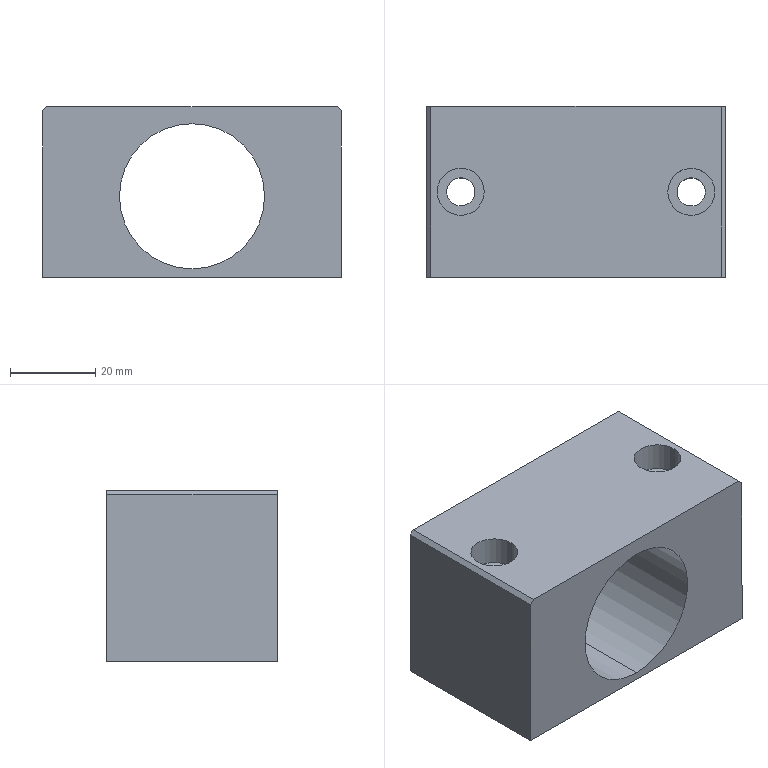Part | SolidWorks | features BaseBody 1 | 1 solid | 36 faces | box 70 x 40 x 40 mm | volume 71369 mm3 | cylinder 18 | plane 10 | cone 8 | commonest cylinder face diameters 4.2 x8 6.6 x4 11 x4 34 x2
STEP:
#1=CARTESIAN_POINT('',(-26.7,157.227,0.));
#2=VERTEX_POINT('',#1);
#3=CARTESIAN_POINT('',(-33.3,157.227,0.));
#4=VERTEX_POINT('',#3);
#5=CARTESIAN_POINT('',(-30.,157.227,0.));
#6=DIRECTION('',(0.,0.,-1.));
#7=DIRECTION('',(1.,0.,0.));
#8=AXIS2_PLACEMENT_3D('',#5,#6,#7);
#9=CIRCLE('',#8,3.3);
#10=EDGE_CURVE('',#2,#4,#9,.T.);
#11=ORIENTED_EDGE('',*,*,#10,.T.);
#12=CARTESIAN_POINT('',(-33.3,157.227,33.2));
#13=VERTEX_POINT('',#12);
#14=CARTESIAN_POINT('',(-33.3,157.227,40.));
#15=DIRECTION('',(0.,0.,1.));
#16=VECTOR('',#15,1000.);
#17=LINE('',#14,#16);
#18=EDGE_CURVE('',#4,#13,#17,.T.);
#19=ORIENTED_EDGE('',*,*,#18,.T.);
#20=CARTESIAN_POINT('',(-26.7,157.227,33.2));
#21=VERTEX_POINT('',#20);
#22=CARTESIAN_POINT('',(-30.,157.227,33.2));
#23=DIRECTION('',(0.,0.,-1.));
#24=DIRECTION('',(1.,0.,0.));
#25=AXIS2_PLACEMENT_3D('',#22,#23,#24);
#26=CIRCLE('',#25,3.3);
#27=EDGE_CURVE('',#21,#13,#26,.T.);
#28=ORIENTED_EDGE('',*,*,#27,.F.);
#29=CARTESIAN_POINT('',(-26.7,157.227,40.));
#30=DIRECTION('',(0.,0.,1.));
#31=VECTOR('',#30,1000.);
#32=LINE('',#29,#31);
#33=EDGE_CURVE('',#2,#21,#32,.T.);
#34=ORIENTED_EDGE('',*,*,#33,.F.);
#35=EDGE_LOOP('',(#11,#19,#28,#34));
#36=FACE_OUTER_BOUND('',#35,.T.);
#37=CARTESIAN_POINT('',(-30.,157.227,40.));
#38=DIRECTION('',(0.,0.,1.));
#39=DIRECTION('',(1.,0.,0.));
#40=AXIS2_PLACEMENT_3D('',#37,#38,#39);
#41=CYLINDRICAL_SURFACE('',#40,3.3);
#42=ADVANCED_FACE('',(#36),#41,.F.);
#43=CARTESIAN_POINT('',(27.3,157.184,0.));
#44=VERTEX_POINT('',#43);
#45=CARTESIAN_POINT('',(20.7,157.184,0.));
#46=VERTEX_POINT('',#45);
#47=CARTESIAN_POINT('',(24.,157.184,0.));
#48=DIRECTION('',(0.,0.,-1.));
#49=DIRECTION('',(1.,0.,0.));
#50=AXIS2_PLACEMENT_3D('',#47,#48,#49);
#51=CIRCLE('',#50,3.3);
#52=EDGE_CURVE('',#44,#46,#51,.T.);
#53=ORIENTED_EDGE('',*,*,#52,.T.);
#54=CARTESIAN_POINT('',(20.7,157.184,33.2));
#55=VERTEX_POINT('',#54);
#56=CARTESIAN_POINT('',(20.7,157.184,40.));
#57=DIRECTION('',(0.,0.,1.));
#58=VECTOR('',#57,1000.);
#59=LINE('',#56,#58);
#60=EDGE_CURVE('',#46,#55,#59,.T.);
#61=ORIENTED_EDGE('',*,*,#60,.T.);
#62=CARTESIAN_POINT('',(27.3,157.184,33.2));
#63=VERTEX_POINT('',#62);
#64=CARTESIAN_POINT('',(24.,157.184,33.2));
#65=DIRECTION('',(0.,0.,-1.));
#66=DIRECTION('',(1.,0.,0.));
#67=AXIS2_PLACEMENT_3D('',#64,#65,#66);
#68=CIRCLE('',#67,3.3);
#69=EDGE_CURVE('',#63,#55,#68,.T.);
#70=ORIENTED_EDGE('',*,*,#69,.F.);
#71=CARTESIAN_POINT('',(27.3,157.184,40.));
#72=DIRECTION('',(0.,0.,1.));
#73=VECTOR('',#72,1000.);
#74=LINE('',#71,#73);
#75=EDGE_CURVE('',#44,#63,#74,.T.);
#76=ORIENTED_EDGE('',*,*,#75,.F.);
#77=EDGE_LOOP('',(#53,#61,#70,#76));
#78=FACE_OUTER_BOUND('',#77,.T.);
#79=CARTESIAN_POINT('',(24.,157.184,40.));
#80=DIRECTION('',(0.,0.,1.));
#81=DIRECTION('',(1.,0.,0.));
#82=AXIS2_PLACEMENT_3D('',#79,#80,#81);
#83=CYLINDRICAL_SURFACE('',#82,3.3);
#84=ADVANCED_FACE('',(#78),#83,.F.);
#85=CARTESIAN_POINT('',(-3.,177.191,2.));
#86=VERTEX_POINT('',#85);
#87=CARTESIAN_POINT('',(-3.,177.191,36.));
#88=VERTEX_POINT('',#87);
#89=CARTESIAN_POINT('',(-3.,177.191,19.));
#90=DIRECTION('',(0.,1.,0.));
#91=DIRECTION('',(0.,0.,-1.));
#92=AXIS2_PLACEMENT_3D('',#89,#90,#91);
#93=CIRCLE('',#92,17.);
#94=EDGE_CURVE('',#86,#88,#93,.T.);
#95=ORIENTED_EDGE('',*,*,#94,.T.);
#96=CARTESIAN_POINT('',(-3.,137.191,36.));
#97=VERTEX_POINT('',#96);
#98=CARTESIAN_POINT('',(-3.,187.191,36.));
#99=DIRECTION('',(0.,-1.,0.));
#100=VECTOR('',#99,1000.);
#101=LINE('',#98,#100);
#102=EDGE_CURVE('',#88,#97,#101,.T.);
#103=ORIENTED_EDGE('',*,*,#102,.T.);
#104=CARTESIAN_POINT('',(-3.,137.191,2.));
#105=VERTEX_POINT('',#104);
#106=CARTESIAN_POINT('',(-3.,137.191,19.));
#107=DIRECTION('',(0.,-1.,0.));
#108=DIRECTION('',(0.,0.,-1.));
#109=AXIS2_PLACEMENT_3D('',#106,#107,#108);
#110=CIRCLE('',#109,17.);
#111=EDGE_CURVE('',#97,#105,#110,.T.);
#112=ORIENTED_EDGE('',*,*,#111,.T.);
#113=CARTESIAN_POINT('',(-3.,187.191,2.));
#114=DIRECTION('',(0.,-1.,0.));
#115=VECTOR('',#114,1000.);
#116=LINE('',#113,#115);
#117=EDGE_CURVE('',#86,#105,#116,.T.);
#118=ORIENTED_EDGE('',*,*,#117,.F.);
#119=EDGE_LOOP('',(#95,#103,#112,#118));
#120=FACE_OUTER_BOUND('',#119,.T.);
#121=CARTESIAN_POINT('',(-3.,187.191,19.));
#122=DIRECTION('',(0.,-1.,0.));
#123=DIRECTION('',(0.,0.,-1.));
#124=AXIS2_PLACEMENT_3D('',#121,#122,#123);
#125=CYLINDRICAL_SURFACE('',#124,17.);
#126=ADVANCED_FACE('',(#120),#125,.F.);
#127=CARTESIAN_POINT('',(-22.486,164.791,28.15));
#128=VERTEX_POINT('',#127);
#129=CARTESIAN_POINT('',(-22.486,164.791,32.35));
#130=VERTEX_POINT('',#129);
#131=CARTESIAN_POINT('',(-22.486,164.791,30.25));
#132=DIRECTION('',(0.,1.,0.));
#133=DIRECTION('',(0.,0.,1.));
#134=AXIS2_PLACEMENT_3D('',#131,#132,#133);
#135=CIRCLE('',#134,2.1);
#136=EDGE_CURVE('',#128,#130,#135,.T.);
#137=ORIENTED_EDGE('',*,*,#136,.F.);
#138=CARTESIAN_POINT('',(-22.486,177.191,28.15));
#139=VERTEX_POINT('',#138);
#140=CARTESIAN_POINT('',(-22.486,177.191,28.15));
#141=DIRECTION('',(0.,1.,0.));
#142=VECTOR('',#141,1000.);
#143=LINE('',#140,#142);
#144=EDGE_CURVE('',#128,#139,#143,.T.);
#145=ORIENTED_EDGE('',*,*,#144,.T.);
#146=CARTESIAN_POINT('',(-22.486,177.191,32.35));
#147=VERTEX_POINT('',#146);
#148=CARTESIAN_POINT('',(-22.486,177.191,30.25));
#149=DIRECTION('',(0.,1.,0.));
#150=DIRECTION('',(0.,0.,1.));
#151=AXIS2_PLACEMENT_3D('',#148,#149,#150);
#152=CIRCLE('',#151,2.1);
#153=EDGE_CURVE('',#139,#147,#152,.T.);
#154=ORIENTED_EDGE('',*,*,#153,.T.);
#155=CARTESIAN_POINT('',(-22.486,177.191,32.35));
#156=DIRECTION('',(0.,1.,0.));
#157=VECTOR('',#156,1000.);
#158=LINE('',#155,#157);
#159=EDGE_CURVE('',#130,#147,#158,.T.);
#160=ORIENTED_EDGE('',*,*,#159,.F.);
#161=EDGE_LOOP('',(#137,#145,#154,#160));
#162=FACE_OUTER_BOUND('',#161,.T.);
#163=CARTESIAN_POINT('',(-22.486,177.191,30.25));
#164=DIRECTION('',(0.,1.,0.));
#165=DIRECTION('',(0.,0.,1.));
#166=AXIS2_PLACEMENT_3D('',#163,#164,#165);
#167=CYLINDRICAL_SURFACE('',#166,2.1);
#168=ADVANCED_FACE('',(#162),#167,.F.);
#169=CARTESIAN_POINT('',(16.486,164.791,28.15));
#170=VERTEX_POINT('',#169);
#171=CARTESIAN_POINT('',(16.486,164.791,32.35));
#172=VERTEX_POINT('',#171);
#173=CARTESIAN_POINT('',(16.486,164.791,30.25));
#174=DIRECTION('',(0.,1.,0.));
#175=DIRECTION('',(0.,0.,1.));
#176=AXIS2_PLACEMENT_3D('',#173,#174,#175);
#177=CIRCLE('',#176,2.1);
#178=EDGE_CURVE('',#170,#172,#177,.T.);
#179=ORIENTED_EDGE('',*,*,#178,.F.);
#180=CARTESIAN_POINT('',(16.486,177.191,28.15));
#181=VERTEX_POINT('',#180);
#182=CARTESIAN_POINT('',(16.486,177.191,28.15));
#183=DIRECTION('',(0.,1.,0.));
#184=VECTOR('',#183,1000.);
#185=LINE('',#182,#184);
#186=EDGE_CURVE('',#170,#181,#185,.T.);
#187=ORIENTED_EDGE('',*,*,#186,.T.);
#188=CARTESIAN_POINT('',(16.486,177.191,32.35));
#189=VERTEX_POINT('',#188);
#190=CARTESIAN_POINT('',(16.486,177.191,30.25));
#191=DIRECTION('',(0.,1.,0.));
#192=DIRECTION('',(0.,0.,1.));
#193=AXIS2_PLACEMENT_3D('',#190,#191,#192);
#194=CIRCLE('',#193,2.1);
#195=EDGE_CURVE('',#181,#189,#194,.T.);
#196=ORIENTED_EDGE('',*,*,#195,.T.);
#197=CARTESIAN_POINT('',(16.486,177.191,32.35));
#198=DIRECTION('',(0.,1.,0.));
#199=VECTOR('',#198,1000.);
#200=LINE('',#197,#199);
#201=EDGE_CURVE('',#172,#189,#200,.T.);
#202=ORIENTED_EDGE('',*,*,#201,.F.);
#203=EDGE_LOOP('',(#179,#187,#196,#202));
#204=FACE_OUTER_BOUND('',#203,.T.);
#205=CARTESIAN_POINT('',(16.486,177.191,30.25));
#206=DIRECTION('',(0.,1.,0.));
#207=DIRECTION('',(0.,0.,1.));
#208=AXIS2_PLACEMENT_3D('',#205,#206,#207);
#209=CYLINDRICAL_SURFACE('',#208,2.1);
#210=ADVANCED_FACE('',(#204),#209,.F.);
#211=CARTESIAN_POINT('',(16.486,164.791,5.65));
#212=VERTEX_POINT('',#211);
#213=CARTESIAN_POINT('',(16.486,164.791,9.85));
#214=VERTEX_POINT('',#213);
#215=CARTESIAN_POINT('',(16.486,164.791,7.75));
#216=DIRECTION('',(0.,1.,0.));
#217=DIRECTION('',(0.,0.,1.));
#218=AXIS2_PLACEMENT_3D('',#215,#216,#217);
#219=CIRCLE('',#218,2.1);
#220=EDGE_CURVE('',#212,#214,#219,.T.);
#221=ORIENTED_EDGE('',*,*,#220,.F.);
#222=CARTESIAN_POINT('',(16.486,177.191,5.65));
#223=VERTEX_POINT('',#222);
#224=CARTESIAN_POINT('',(16.486,177.191,5.65));
#225=DIRECTION('',(0.,1.,0.));
#226=VECTOR('',#225,1000.);
#227=LINE('',#224,#226);
#228=EDGE_CURVE('',#212,#223,#227,.T.);
#229=ORIENTED_EDGE('',*,*,#228,.T.);
#230=CARTESIAN_POINT('',(16.486,177.191,9.85));
#231=VERTEX_POINT('',#230);
#232=CARTESIAN_POINT('',(16.486,177.191,7.75));
#233=DIRECTION('',(0.,1.,0.));
#234=DIRECTION('',(0.,0.,1.));
#235=AXIS2_PLACEMENT_3D('',#232,#233,#234);
#236=CIRCLE('',#235,2.1);
#237=EDGE_CURVE('',#223,#231,#236,.T.);
#238=ORIENTED_EDGE('',*,*,#237,.T.);
#239=CARTESIAN_POINT('',(16.486,177.191,9.85));
#240=DIRECTION('',(0.,1.,0.));
#241=VECTOR('',#240,1000.);
#242=LINE('',#239,#241);
#243=EDGE_CURVE('',#214,#231,#242,.T.);
#244=ORIENTED_EDGE('',*,*,#243,.F.);
#245=EDGE_LOOP('',(#221,#229,#238,#244));
#246=FACE_OUTER_BOUND('',#245,.T.);
#247=CARTESIAN_POINT('',(16.486,177.191,7.75));
#248=DIRECTION('',(0.,1.,0.));
#249=DIRECTION('',(0.,0.,1.));
#250=AXIS2_PLACEMENT_3D('',#247,#248,#249);
#251=CYLINDRICAL_SURFACE('',#250,2.1);
#252=ADVANCED_FACE('',(#246),#251,.F.);
#253=CARTESIAN_POINT('',(-22.486,164.791,5.65));
#254=VERTEX_POINT('',#253);
#255=CARTESIAN_POINT('',(-22.486,164.791,9.85));
#256=VERTEX_POINT('',#255);
#257=CARTESIAN_POINT('',(-22.486,164.791,7.75));
#258=DIRECTION('',(0.,1.,0.));
#259=DIRECTION('',(0.,0.,1.));
#260=AXIS2_PLACEMENT_3D('',#257,#258,#259);
#261=CIRCLE('',#260,2.1);
#262=EDGE_CURVE('',#254,#256,#261,.T.);
#263=ORIENTED_EDGE('',*,*,#262,.F.);
#264=CARTESIAN_POINT('',(-22.486,177.191,5.65));
#265=VERTEX_POINT('',#264);
#266=CARTESIAN_POINT('',(-22.486,177.191,5.65));
#267=DIRECTION('',(0.,1.,0.));
#268=VECTOR('',#267,1000.);
#269=LINE('',#266,#268);
#270=EDGE_CURVE('',#254,#265,#269,.T.);
#271=ORIENTED_EDGE('',*,*,#270,.T.);
#272=CARTESIAN_POINT('',(-22.486,177.191,9.85));
#273=VERTEX_POINT('',#272);
#274=CARTESIAN_POINT('',(-22.486,177.191,7.75));
#275=DIRECTION('',(0.,1.,0.));
#276=DIRECTION('',(0.,0.,1.));
#277=AXIS2_PLACEMENT_3D('',#274,#275,#276);
#278=CIRCLE('',#277,2.1);
#279=EDGE_CURVE('',#265,#273,#278,.T.);
#280=ORIENTED_EDGE('',*,*,#279,.T.);
#281=CARTESIAN_POINT('',(-22.486,177.191,9.85));
#282=DIRECTION('',(0.,1.,0.));
#283=VECTOR('',#282,1000.);
#284=LINE('',#281,#283);
#285=EDGE_CURVE('',#256,#273,#284,.T.);
#286=ORIENTED_EDGE('',*,*,#285,.F.);
#287=EDGE_LOOP('',(#263,#271,#280,#286));
#288=FACE_OUTER_BOUND('',#287,.T.);
#289=CARTESIAN_POINT('',(-22.486,177.191,7.75));
#290=DIRECTION('',(0.,1.,0.));
#291=DIRECTION('',(0.,0.,1.));
#292=AXIS2_PLACEMENT_3D('',#289,#290,#291);
#293=CYLINDRICAL_SURFACE('',#292,2.1);
#294=ADVANCED_FACE('',(#288),#293,.F.);
#295=CARTESIAN_POINT('',(-24.5,157.227,33.2));
#296=VERTEX_POINT('',#295);
#297=CARTESIAN_POINT('',(-35.5,157.227,33.2));
#298=VERTEX_POINT('',#297);
#299=CARTESIAN_POINT('',(-30.,157.227,33.2));
#300=DIRECTION('',(0.,0.,-1.));
#301=DIRECTION('',(1.,0.,0.));
#302=AXIS2_PLACEMENT_3D('',#299,#300,#301);
#303=CIRCLE('',#302,5.5);
#304=EDGE_CURVE('',#296,#298,#303,.T.);
#305=ORIENTED_EDGE('',*,*,#304,.T.);
#306=CARTESIAN_POINT('',(-35.5,157.227,40.));
#307=VERTEX_POINT('',#306);
#308=CARTESIAN_POINT('',(-35.5,157.227,40.));
#309=DIRECTION('',(0.,0.,1.));
#310=VECTOR('',#309,1000.);
#311=LINE('',#308,#310);
#312=EDGE_CURVE('',#298,#307,#311,.T.);
#313=ORIENTED_EDGE('',*,*,#312,.T.);
#314=CARTESIAN_POINT('',(-24.5,157.227,40.));
#315=VERTEX_POINT('',#314);
#316=CARTESIAN_POINT('',(-30.,157.227,40.));
#317=DIRECTION('',(0.,0.,-1.));
#318=DIRECTION('',(1.,0.,0.));
#319=AXIS2_PLACEMENT_3D('',#316,#317,#318);
#320=CIRCLE('',#319,5.5);
#321=EDGE_CURVE('',#315,#307,#320,.T.);
#322=ORIENTED_EDGE('',*,*,#321,.F.);
#323=CARTESIAN_POINT('',(-24.5,157.227,40.));
#324=DIRECTION('',(0.,0.,1.));
#325=VECTOR('',#324,1000.);
#326=LINE('',#323,#325);
#327=EDGE_CURVE('',#296,#315,#326,.T.);
#328=ORIENTED_EDGE('',*,*,#327,.F.);
#329=EDGE_LOOP('',(#305,#313,#322,#328));
#330=FACE_OUTER_BOUND('',#329,.T.);
#331=CARTESIAN_POINT('',(-30.,157.227,40.));
#332=DIRECTION('',(0.,0.,1.));
#333=DIRECTION('',(1.,0.,0.));
#334=AXIS2_PLACEMENT_3D('',#331,#332,#333);
#335=CYLINDRICAL_SURFACE('',#334,5.5);
#336=ADVANCED_FACE('',(#330),#335,.F.);
#337=CARTESIAN_POINT('',(29.5,157.184,33.2));
#338=VERTEX_POINT('',#337);
#339=CARTESIAN_POINT('',(18.5,157.184,33.2));
#340=VERTEX_POINT('',#339);
#341=CARTESIAN_POINT('',(24.,157.184,33.2));
#342=DIRECTION('',(0.,0.,-1.));
#343=DIRECTION('',(1.,0.,0.));
#344=AXIS2_PLACEMENT_3D('',#341,#342,#343);
#345=CIRCLE('',#344,5.5);
#346=EDGE_CURVE('',#338,#340,#345,.T.);
#347=ORIENTED_EDGE('',*,*,#346,.T.);
#348=CARTESIAN_POINT('',(18.5,157.184,40.));
#349=VERTEX_POINT('',#348);
#350=CARTESIAN_POINT('',(18.5,157.184,40.));
#351=DIRECTION('',(0.,0.,1.));
#352=VECTOR('',#351,1000.);
#353=LINE('',#350,#352);
#354=EDGE_CURVE('',#340,#349,#353,.T.);
#355=ORIENTED_EDGE('',*,*,#354,.T.);
#356=CARTESIAN_POINT('',(29.5,157.184,40.));
#357=VERTEX_POINT('',#356);
#358=CARTESIAN_POINT('',(24.,157.184,40.));
#359=DIRECTION('',(0.,0.,-1.));
#360=DIRECTION('',(1.,0.,0.));
#361=AXIS2_PLACEMENT_3D('',#358,#359,#360);
#362=CIRCLE('',#361,5.5);
#363=EDGE_CURVE('',#357,#349,#362,.T.);
#364=ORIENTED_EDGE('',*,*,#363,.F.);
#365=CARTESIAN_POINT('',(29.5,157.184,40.));
#366=DIRECTION('',(0.,0.,1.));
#367=VECTOR('',#366,1000.);
#368=LINE('',#365,#367);
#369=EDGE_CURVE('',#338,#357,#368,.T.);
#370=ORIENTED_EDGE('',*,*,#369,.F.);
#371=EDGE_LOOP('',(#347,#355,#364,#370));
#372=FACE_OUTER_BOUND('',#371,.T.);
#373=CARTESIAN_POINT('',(24.,157.184,40.));
#374=DIRECTION('',(0.,0.,1.));
#375=DIRECTION('',(1.,0.,0.));
#376=AXIS2_PLACEMENT_3D('',#373,#374,#375);
#377=CYLINDRICAL_SURFACE('',#376,5.5);
#378=ADVANCED_FACE('',(#372),#377,.F.);
#379=CARTESIAN_POINT('',(-22.486,163.53,30.25));
#380=VERTEX_POINT('',#379);
#381=CARTESIAN_POINT('',(-22.486,164.791,32.35));
#382=DIRECTION('',(0.,0.515,0.8572));
#383=VECTOR('',#382,1000.);
#384=LINE('',#381,#383);
#385=EDGE_CURVE('',#380,#130,#384,.T.);
#386=ORIENTED_EDGE('',*,*,#385,.F.);
#387=CARTESIAN_POINT('',(-22.486,164.791,28.15));
#388=DIRECTION('',(0.,0.515,-0.8572));
#389=VECTOR('',#388,1000.);
#390=LINE('',#387,#389);
#391=EDGE_CURVE('',#380,#128,#390,.T.);
#392=ORIENTED_EDGE('',*,*,#391,.T.);
#393=ORIENTED_EDGE('',*,*,#136,.T.);
#394=EDGE_LOOP('',(#386,#392,#393));
#395=FACE_OUTER_BOUND('',#394,.T.);
#396=CARTESIAN_POINT('',(-22.486,164.791,30.25));
#397=DIRECTION('',(0.,1.,0.));
#398=DIRECTION('',(0.,0.,1.));
#399=AXIS2_PLACEMENT_3D('',#396,#397,#398);
#400=CONICAL_SURFACE('',#399,2.1,1.03);
#401=ADVANCED_FACE('',(#395),#400,.F.);
#402=CARTESIAN_POINT('',(16.486,163.53,30.25));
#403=VERTEX_POINT('',#402);
#404=CARTESIAN_POINT('',(16.486,164.791,32.35));
#405=DIRECTION('',(0.,0.515,0.8572));
#406=VECTOR('',#405,1000.);
#407=LINE('',#404,#406);
#408=EDGE_CURVE('',#403,#172,#407,.T.);
#409=ORIENTED_EDGE('',*,*,#408,.F.);
#410=CARTESIAN_POINT('',(16.486,164.791,28.15));
#411=DIRECTION('',(0.,0.515,-0.8572));
#412=VECTOR('',#411,1000.);
#413=LINE('',#410,#412);
#414=EDGE_CURVE('',#403,#170,#413,.T.);
#415=ORIENTED_EDGE('',*,*,#414,.T.);
#416=ORIENTED_EDGE('',*,*,#178,.T.);
#417=EDGE_LOOP('',(#409,#415,#416));
#418=FACE_OUTER_BOUND('',#417,.T.);
#419=CARTESIAN_POINT('',(16.486,164.791,30.25));
#420=DIRECTION('',(0.,1.,0.));
#421=DIRECTION('',(0.,0.,1.));
#422=AXIS2_PLACEMENT_3D('',#419,#420,#421);
#423=CONICAL_SURFACE('',#422,2.1,1.03);
#424=ADVANCED_FACE('',(#418),#423,.F.);
#425=CARTESIAN_POINT('',(16.486,163.53,7.75));
#426=VERTEX_POINT('',#425);
#427=CARTESIAN_POINT('',(16.486,164.791,9.85));
#428=DIRECTION('',(0.,0.515,0.8572));
#429=VECTOR('',#428,1000.);
#430=LINE('',#427,#429);
#431=EDGE_CURVE('',#426,#214,#430,.T.);
#432=ORIENTED_EDGE('',*,*,#431,.F.);
#433=CARTESIAN_POINT('',(16.486,164.791,5.65));
#434=DIRECTION('',(0.,0.515,-0.8572));
#435=VECTOR('',#434,1000.);
#436=LINE('',#433,#435);
#437=EDGE_CURVE('',#426,#212,#436,.T.);
#438=ORIENTED_EDGE('',*,*,#437,.T.);
#439=ORIENTED_EDGE('',*,*,#220,.T.);
#440=EDGE_LOOP('',(#432,#438,#439));
#441=FACE_OUTER_BOUND('',#440,.T.);
#442=CARTESIAN_POINT('',(16.486,164.791,7.75));
#443=DIRECTION('',(0.,1.,0.));
#444=DIRECTION('',(0.,0.,1.));
#445=AXIS2_PLACEMENT_3D('',#442,#443,#444);
#446=CONICAL_SURFACE('',#445,2.1,1.03);
#447=ADVANCED_FACE('',(#441),#446,.F.);
#448=CARTESIAN_POINT('',(-22.486,163.53,7.75));
#449=VERTEX_POINT('',#448);
#450=CARTESIAN_POINT('',(-22.486,164.791,9.85));
#451=DIRECTION('',(0.,0.515,0.8572));
#452=VECTOR('',#451,1000.);
#453=LINE('',#450,#452);
#454=EDGE_CURVE('',#449,#256,#453,.T.);
#455=ORIENTED_EDGE('',*,*,#454,.F.);
#456=CARTESIAN_POINT('',(-22.486,164.791,5.65));
#457=DIRECTION('',(0.,0.515,-0.8572));
#458=VECTOR('',#457,1000.);
#459=LINE('',#456,#458);
#460=EDGE_CURVE('',#449,#254,#459,.T.);
#461=ORIENTED_EDGE('',*,*,#460,.T.);
#462=ORIENTED_EDGE('',*,*,#262,.T.);
#463=EDGE_LOOP('',(#455,#461,#462));
#464=FACE_OUTER_BOUND('',#463,.T.);
#465=CARTESIAN_POINT('',(-22.486,164.791,7.75));
#466=DIRECTION('',(0.,1.,0.));
#467=DIRECTION('',(0.,0.,1.));
#468=AXIS2_PLACEMENT_3D('',#465,#466,#467);
#469=CONICAL_SURFACE('',#468,2.1,1.03);
#470=ADVANCED_FACE('',(#464),#469,.F.);
#471=CARTESIAN_POINT('',(-38.,137.191,0.));
#472=VERTEX_POINT('',#471);
#473=CARTESIAN_POINT('',(32.,137.191,0.));
#474=VERTEX_POINT('',#473);
#475=CARTESIAN_POINT('',(0.,137.191,0.));
#476=DIRECTION('',(1.,0.,0.));
#477=VECTOR('',#476,1000.);
#478=LINE('',#475,#477);
#479=EDGE_CURVE('',#472,#474,#478,.T.);
#480=ORIENTED_EDGE('',*,*,#479,.F.);
#481=CARTESIAN_POINT('',(-38.,177.191,0.));
#482=VERTEX_POINT('',#481);
#483=CARTESIAN_POINT('',(-38.,0.,0.));
#484=DIRECTION('',(0.,-1.,0.));
#485=VECTOR('',#484,1000.);
#486=LINE('',#483,#485);
#487=EDGE_CURVE('',#482,#472,#486,.T.);
#488=ORIENTED_EDGE('',*,*,#487,.F.);
#489=CARTESIAN_POINT('',(32.,177.191,0.));
#490=VERTEX_POINT('',#489);
#491=CARTESIAN_POINT('',(0.,177.191,0.));
#492=DIRECTION('',(-1.,0.,0.));
#493=VECTOR('',#492,1000.);
#494=LINE('',#491,#493);
#495=EDGE_CURVE('',#490,#482,#494,.T.);
#496=ORIENTED_EDGE('',*,*,#495,.F.);
#497=CARTESIAN_POINT('',(32.,0.,0.));
#498=DIRECTION('',(0.,1.,0.));
#499=VECTOR('',#498,1000.);
#500=LINE('',#497,#499);
#501=EDGE_CURVE('',#474,#490,#500,.T.);
#502=ORIENTED_EDGE('',*,*,#501,.F.);
#503=EDGE_LOOP('',(#480,#488,#496,#502));
#504=FACE_OUTER_BOUND('',#503,.T.);
#505=ORIENTED_EDGE('',*,*,#10,.F.);
#506=CARTESIAN_POINT('',(-30.,157.227,0.));
#507=DIRECTION('',(0.,0.,-1.));
#508=DIRECTION('',(1.,0.,0.));
#509=AXIS2_PLACEMENT_3D('',#506,#507,#508);
#510=CIRCLE('',#509,3.3);
#511=EDGE_CURVE('',#4,#2,#510,.T.);
#512=ORIENTED_EDGE('',*,*,#511,.F.);
#513=EDGE_LOOP('',(#505,#512));
#514=FACE_BOUND('',#513,.T.);
#515=ORIENTED_EDGE('',*,*,#52,.F.);
#516=CARTESIAN_POINT('',(24.,157.184,0.));
#517=DIRECTION('',(0.,0.,-1.));
#518=DIRECTION('',(1.,0.,0.));
#519=AXIS2_PLACEMENT_3D('',#516,#517,#518);
#520=CIRCLE('',#519,3.3);
#521=EDGE_CURVE('',#46,#44,#520,.T.);
#522=ORIENTED_EDGE('',*,*,#521,.F.);
#523=EDGE_LOOP('',(#515,#522));
#524=FACE_BOUND('',#523,.T.);
#525=CARTESIAN_POINT('',(0.,0.,0.));
#526=DIRECTION('',(0.,0.,1.));
#527=DIRECTION('',(1.,0.,0.));
#528=AXIS2_PLACEMENT_3D('',#525,#526,#527);
#529=PLANE('',#528);
#530=ADVANCED_FACE('',(#504,#514,#524),#529,.F.);
#531=CARTESIAN_POINT('',(32.,137.191,39.));
#532=VERTEX_POINT('',#531);
#533=CARTESIAN_POINT('',(32.,177.191,39.));
#534=VERTEX_POINT('',#533);
#535=CARTESIAN_POINT('',(32.,137.191,39.));
#536=DIRECTION('',(0.,1.,0.));
#537=VECTOR('',#536,1000.);
#538=LINE('',#535,#537);
#539=EDGE_CURVE('',#532,#534,#538,.T.);
#540=ORIENTED_EDGE('',*,*,#539,.F.);
#541=CARTESIAN_POINT('',(32.,137.191,40.));
#542=DIRECTION('',(0.,0.,1.));
#543=VECTOR('',#542,1000.);
#544=LINE('',#541,#543);
#545=EDGE_CURVE('',#474,#532,#544,.T.);
#546=ORIENTED_EDGE('',*,*,#545,.F.);
#547=ORIENTED_EDGE('',*,*,#501,.T.);
#548=CARTESIAN_POINT('',(32.,177.191,40.));
#549=DIRECTION('',(0.,0.,-1.));
#550=VECTOR('',#549,1000.);
#551=LINE('',#548,#550);
#552=EDGE_CURVE('',#534,#490,#551,.T.);
#553=ORIENTED_EDGE('',*,*,#552,.F.);
#554=EDGE_LOOP('',(#540,#546,#547,#553));
#555=FACE_OUTER_BOUND('',#554,.T.);
#556=CARTESIAN_POINT('',(32.,137.191,40.));
#557=DIRECTION('',(-1.,0.,0.));
#558=DIRECTION('',(0.,0.,1.));
#559=AXIS2_PLACEMENT_3D('',#556,#557,#558);
#560=PLANE('',#559);
#561=ADVANCED_FACE('',(#555),#560,.F.);
#562=CARTESIAN_POINT('',(-38.,137.191,39.));
#563=VERTEX_POINT('',#562);
#564=CARTESIAN_POINT('',(-37.,137.191,40.));
#565=VERTEX_POINT('',#564);
#566=CARTESIAN_POINT('',(-37.,137.191,40.));
#567=DIRECTION('',(0.7071,0.,0.7071));
#568=VECTOR('',#567,1000.);
#569=LINE('',#566,#568);
#570=EDGE_CURVE('',#563,#565,#569,.T.);
#571=ORIENTED_EDGE('',*,*,#570,.F.);
#572=CARTESIAN_POINT('',(-38.,137.191,40.));
#573=DIRECTION('',(0.,0.,1.));
#574=VECTOR('',#573,1000.);
#575=LINE('',#572,#574);
#576=EDGE_CURVE('',#472,#563,#575,.T.);
#577=ORIENTED_EDGE('',*,*,#576,.F.);
#578=ORIENTED_EDGE('',*,*,#479,.T.);
#579=ORIENTED_EDGE('',*,*,#545,.T.);
#580=CARTESIAN_POINT('',(31.,137.191,40.));
#581=VERTEX_POINT('',#580);
#582=CARTESIAN_POINT('',(31.,137.191,40.));
#583=DIRECTION('',(0.7071,0.,-0.7071));
#584=VECTOR('',#583,1000.);
#585=LINE('',#582,#584);
#586=EDGE_CURVE('',#581,#532,#585,.T.);
#587=ORIENTED_EDGE('',*,*,#586,.F.);
#588=CARTESIAN_POINT('',(32.,137.191,40.));
#589=DIRECTION('',(1.,0.,0.));
#590=VECTOR('',#589,1000.);
#591=LINE('',#588,#590);
#592=EDGE_CURVE('',#565,#581,#591,.T.);
#593=ORIENTED_EDGE('',*,*,#592,.F.);
#594=EDGE_LOOP('',(#571,#577,#578,#579,#587,#593));
#595=FACE_OUTER_BOUND('',#594,.T.);
#596=CARTESIAN_POINT('',(-3.,137.191,19.));
#597=DIRECTION('',(0.,-1.,0.));
#598=DIRECTION('',(0.,0.,-1.));
#599=AXIS2_PLACEMENT_3D('',#596,#597,#598);
#600=CIRCLE('',#599,17.);
#601=EDGE_CURVE('',#105,#97,#600,.T.);
#602=ORIENTED_EDGE('',*,*,#601,.F.);
#603=ORIENTED_EDGE('',*,*,#111,.F.);
#604=EDGE_LOOP('',(#602,#603));
#605=FACE_BOUND('',#604,.T.);
#606=CARTESIAN_POINT('',(32.,137.191,40.));
#607=DIRECTION('',(0.,1.,0.));
#608=DIRECTION('',(-1.,0.,0.));
#609=AXIS2_PLACEMENT_3D('',#606,#607,#608);
#610=PLANE('',#609);
#611=ADVANCED_FACE('',(#595,#605),#610,.F.);
#612=CARTESIAN_POINT('',(-38.,177.191,39.));
#613=VERTEX_POINT('',#612);
#614=CARTESIAN_POINT('',(-38.,137.191,39.));
#615=DIRECTION('',(0.,-1.,0.));
#616=VECTOR('',#615,1000.);
#617=LINE('',#614,#616);
#618=EDGE_CURVE('',#613,#563,#617,.T.);
#619=ORIENTED_EDGE('',*,*,#618,.F.);
#620=CARTESIAN_POINT('',(-38.,177.191,40.));
#621=DIRECTION('',(0.,0.,1.));
#622=VECTOR('',#621,1000.);
#623=LINE('',#620,#622);
#624=EDGE_CURVE('',#482,#613,#623,.T.);
#625=ORIENTED_EDGE('',*,*,#624,.F.);
#626=ORIENTED_EDGE('',*,*,#487,.T.);
#627=ORIENTED_EDGE('',*,*,#576,.T.);
#628=EDGE_LOOP('',(#619,#625,#626,#627));
#629=FACE_OUTER_BOUND('',#628,.T.);
#630=CARTESIAN_POINT('',(-38.,137.191,40.));
#631=DIRECTION('',(1.,0.,0.));
#632=DIRECTION('',(0.,0.,-1.));
#633=AXIS2_PLACEMENT_3D('',#630,#631,#632);
#634=PLANE('',#633);
#635=ADVANCED_FACE('',(#629),#634,.F.);
#636=CARTESIAN_POINT('',(-37.,177.191,40.));
#637=VERTEX_POINT('',#636);
#638=CARTESIAN_POINT('',(-37.,177.191,40.));
#639=DIRECTION('',(-0.7071,0.,-0.7071));
#640=VECTOR('',#639,1000.);
#641=LINE('',#638,#640);
#642=EDGE_CURVE('',#637,#613,#641,.T.);
#643=ORIENTED_EDGE('',*,*,#642,.F.);
#644=CARTESIAN_POINT('',(31.,177.191,40.));
#645=VERTEX_POINT('',#644);
#646=CARTESIAN_POINT('',(32.,177.191,40.));
#647=DIRECTION('',(-1.,0.,0.));
#648=VECTOR('',#647,1000.);
#649=LINE('',#646,#648);
#650=EDGE_CURVE('',#645,#637,#649,.T.);
#651=ORIENTED_EDGE('',*,*,#650,.F.);
#652=CARTESIAN_POINT('',(32.,177.191,39.));
#653=DIRECTION('',(-0.7071,0.,0.7071));
#654=VECTOR('',#653,1000.);
#655=LINE('',#652,#654);
#656=EDGE_CURVE('',#534,#645,#655,.T.);
#657=ORIENTED_EDGE('',*,*,#656,.F.);
#658=ORIENTED_EDGE('',*,*,#552,.T.);
#659=ORIENTED_EDGE('',*,*,#495,.T.);
#660=ORIENTED_EDGE('',*,*,#624,.T.);
#661=EDGE_LOOP('',(#643,#651,#657,#658,#659,#660));
#662=FACE_OUTER_BOUND('',#661,.T.);
#663=ORIENTED_EDGE('',*,*,#94,.F.);
#664=CARTESIAN_POINT('',(-3.,177.191,19.));
#665=DIRECTION('',(0.,1.,0.));
#666=DIRECTION('',(0.,0.,-1.));
#667=AXIS2_PLACEMENT_3D('',#664,#665,#666);
#668=CIRCLE('',#667,17.);
#669=EDGE_CURVE('',#88,#86,#668,.T.);
#670=ORIENTED_EDGE('',*,*,#669,.F.);
#671=EDGE_LOOP('',(#663,#670));
#672=FACE_BOUND('',#671,.T.);
#673=CARTESIAN_POINT('',(-22.486,177.191,30.25));
#674=DIRECTION('',(0.,1.,0.));
#675=DIRECTION('',(0.,0.,1.));
#676=AXIS2_PLACEMENT_3D('',#673,#674,#675);
#677=CIRCLE('',#676,2.1);
#678=EDGE_CURVE('',#147,#139,#677,.T.);
#679=ORIENTED_EDGE('',*,*,#678,.F.);
#680=ORIENTED_EDGE('',*,*,#153,.F.);
#681=EDGE_LOOP('',(#679,#680));
#682=FACE_BOUND('',#681,.T.);
#683=CARTESIAN_POINT('',(16.486,177.191,30.25));
#684=DIRECTION('',(0.,1.,0.));
#685=DIRECTION('',(0.,0.,1.));
#686=AXIS2_PLACEMENT_3D('',#683,#684,#685);
#687=CIRCLE('',#686,2.1);
#688=EDGE_CURVE('',#189,#181,#687,.T.);
#689=ORIENTED_EDGE('',*,*,#688,.F.);
#690=ORIENTED_EDGE('',*,*,#195,.F.);
#691=EDGE_LOOP('',(#689,#690));
#692=FACE_BOUND('',#691,.T.);
#693=CARTESIAN_POINT('',(16.486,177.191,7.75));
#694=DIRECTION('',(0.,1.,0.));
#695=DIRECTION('',(0.,0.,1.));
#696=AXIS2_PLACEMENT_3D('',#693,#694,#695);
#697=CIRCLE('',#696,2.1);
#698=EDGE_CURVE('',#231,#223,#697,.T.);
#699=ORIENTED_EDGE('',*,*,#698,.F.);
#700=ORIENTED_EDGE('',*,*,#237,.F.);
#701=EDGE_LOOP('',(#699,#700));
#702=FACE_BOUND('',#701,.T.);
#703=CARTESIAN_POINT('',(-22.486,177.191,7.75));
#704=DIRECTION('',(0.,1.,0.));
#705=DIRECTION('',(0.,0.,1.));
#706=AXIS2_PLACEMENT_3D('',#703,#704,#705);
#707=CIRCLE('',#706,2.1);
#708=EDGE_CURVE('',#273,#265,#707,.T.);
#709=ORIENTED_EDGE('',*,*,#708,.F.);
#710=ORIENTED_EDGE('',*,*,#279,.F.);
#711=EDGE_LOOP('',(#709,#710));
#712=FACE_BOUND('',#711,.T.);
#713=CARTESIAN_POINT('',(32.,177.191,40.));
#714=DIRECTION('',(0.,-1.,0.));
#715=DIRECTION('',(1.,0.,0.));
#716=AXIS2_PLACEMENT_3D('',#713,#714,#715);
#717=PLANE('',#716);
#718=ADVANCED_FACE('',(#662,#672,#682,#692,#702,#712),#717,.F.);
#719=ORIENTED_EDGE('',*,*,#18,.F.);
#720=ORIENTED_EDGE('',*,*,#511,.T.);
#721=ORIENTED_EDGE('',*,*,#33,.T.);
#722=CARTESIAN_POINT('',(-30.,157.227,33.2));
#723=DIRECTION('',(0.,0.,-1.));
#724=DIRECTION('',(1.,0.,0.));
#725=AXIS2_PLACEMENT_3D('',#722,#723,#724);
#726=CIRCLE('',#725,3.3);
#727=EDGE_CURVE('',#13,#21,#726,.T.);
#728=ORIENTED_EDGE('',*,*,#727,.F.);
#729=EDGE_LOOP('',(#719,#720,#721,#728));
#730=FACE_OUTER_BOUND('',#729,.T.);
#731=CARTESIAN_POINT('',(-30.,157.227,40.));
#732=DIRECTION('',(0.,0.,1.));
#733=DIRECTION('',(1.,0.,0.));
#734=AXIS2_PLACEMENT_3D('',#731,#732,#733);
#735=CYLINDRICAL_SURFACE('',#734,3.3);
#736=ADVANCED_FACE('',(#730),#735,.F.);
#737=ORIENTED_EDGE('',*,*,#60,.F.);
#738=ORIENTED_EDGE('',*,*,#521,.T.);
#739=ORIENTED_EDGE('',*,*,#75,.T.);
#740=CARTESIAN_POINT('',(24.,157.184,33.2));
#741=DIRECTION('',(0.,0.,-1.));
#742=DIRECTION('',(1.,0.,0.));
#743=AXIS2_PLACEMENT_3D('',#740,#741,#742);
#744=CIRCLE('',#743,3.3);
#745=EDGE_CURVE('',#55,#63,#744,.T.);
#746=ORIENTED_EDGE('',*,*,#745,.F.);
#747=EDGE_LOOP('',(#737,#738,#739,#746));
#748=FACE_OUTER_BOUND('',#747,.T.);
#749=CARTESIAN_POINT('',(24.,157.184,40.));
#750=DIRECTION('',(0.,0.,1.));
#751=DIRECTION('',(1.,0.,0.));
#752=AXIS2_PLACEMENT_3D('',#749,#750,#751);
#753=CYLINDRICAL_SURFACE('',#752,3.3);
#754=ADVANCED_FACE('',(#748),#753,.F.);
#755=ORIENTED_EDGE('',*,*,#656,.T.);
#756=CARTESIAN_POINT('',(31.,0.,40.));
#757=DIRECTION('',(0.,-1.,0.));
#758=VECTOR('',#757,1000.);
#759=LINE('',#756,#758);
#760=EDGE_CURVE('',#645,#581,#759,.T.);
#761=ORIENTED_EDGE('',*,*,#760,.T.);
#762=ORIENTED_EDGE('',*,*,#586,.T.);
#763=ORIENTED_EDGE('',*,*,#539,.T.);
#764=EDGE_LOOP('',(#755,#761,#762,#763));
#765=FACE_OUTER_BOUND('',#764,.T.);
#766=CARTESIAN_POINT('',(31.,0.,40.));
#767=DIRECTION('',(0.7071,0.,0.7071));
#768=DIRECTION('',(0.7071,0.,-0.7071));
#769=AXIS2_PLACEMENT_3D('',#766,#767,#768);
#770=PLANE('',#769);
#771=ADVANCED_FACE('',(#765),#770,.T.);
#772=ORIENTED_EDGE('',*,*,#592,.T.);
#773=ORIENTED_EDGE('',*,*,#760,.F.);
#774=ORIENTED_EDGE('',*,*,#650,.T.);
#775=CARTESIAN_POINT('',(-37.,0.,40.));
#776=DIRECTION('',(0.,-1.,0.));
#777=VECTOR('',#776,1000.);
#778=LINE('',#775,#777);
#779=EDGE_CURVE('',#637,#565,#778,.T.);
#780=ORIENTED_EDGE('',*,*,#779,.T.);
#781=EDGE_LOOP('',(#772,#773,#774,#780));
#782=FACE_OUTER_BOUND('',#781,.T.);
#783=ORIENTED_EDGE('',*,*,#321,.T.);
#784=CARTESIAN_POINT('',(-30.,157.227,40.));
#785=DIRECTION('',(0.,0.,-1.));
#786=DIRECTION('',(1.,0.,0.));
#787=AXIS2_PLACEMENT_3D('',#784,#785,#786);
#788=CIRCLE('',#787,5.5);
#789=EDGE_CURVE('',#307,#315,#788,.T.);
#790=ORIENTED_EDGE('',*,*,#789,.T.);
#791=EDGE_LOOP('',(#783,#790));
#792=FACE_BOUND('',#791,.T.);
#793=ORIENTED_EDGE('',*,*,#363,.T.);
#794=CARTESIAN_POINT('',(24.,157.184,40.));
#795=DIRECTION('',(0.,0.,-1.));
#796=DIRECTION('',(1.,0.,0.));
#797=AXIS2_PLACEMENT_3D('',#794,#795,#796);
#798=CIRCLE('',#797,5.5);
#799=EDGE_CURVE('',#349,#357,#798,.T.);
#800=ORIENTED_EDGE('',*,*,#799,.T.);
#801=EDGE_LOOP('',(#793,#800));
#802=FACE_BOUND('',#801,.T.);
#803=CARTESIAN_POINT('',(0.,0.,40.));
#804=DIRECTION('',(0.,0.,1.));
#805=DIRECTION('',(1.,0.,0.));
#806=AXIS2_PLACEMENT_3D('',#803,#804,#805);
#807=PLANE('',#806);
#808=ADVANCED_FACE('',(#782,#792,#802),#807,.T.);
#809=ORIENTED_EDGE('',*,*,#102,.F.);
#810=ORIENTED_EDGE('',*,*,#669,.T.);
#811=ORIENTED_EDGE('',*,*,#117,.T.);
#812=ORIENTED_EDGE('',*,*,#601,.T.);
#813=EDGE_LOOP('',(#809,#810,#811,#812));
#814=FACE_OUTER_BOUND('',#813,.T.);
#815=CARTESIAN_POINT('',(-3.,187.191,19.));
#816=DIRECTION('',(0.,-1.,0.));
#817=DIRECTION('',(0.,0.,-1.));
#818=AXIS2_PLACEMENT_3D('',#815,#816,#817);
#819=CYLINDRICAL_SURFACE('',#818,17.);
#820=ADVANCED_FACE('',(#814),#819,.F.);
#821=ORIENTED_EDGE('',*,*,#570,.T.);
#822=ORIENTED_EDGE('',*,*,#779,.F.);
#823=ORIENTED_EDGE('',*,*,#642,.T.);
#824=ORIENTED_EDGE('',*,*,#618,.T.);
#825=EDGE_LOOP('',(#821,#822,#823,#824));
#826=FACE_OUTER_BOUND('',#825,.T.);
#827=CARTESIAN_POINT('',(-37.,0.,40.));
#828=DIRECTION('',(-0.7071,0.,0.7071));
#829=DIRECTION('',(0.7071,0.,0.7071));
#830=AXIS2_PLACEMENT_3D('',#827,#828,#829);
#831=PLANE('',#830);
#832=ADVANCED_FACE('',(#826),#831,.T.);
#833=ORIENTED_EDGE('',*,*,#144,.F.);
#834=CARTESIAN_POINT('',(-22.486,164.791,30.25));
#835=DIRECTION('',(0.,1.,0.));
#836=DIRECTION('',(0.,0.,1.));
#837=AXIS2_PLACEMENT_3D('',#834,#835,#836);
#838=CIRCLE('',#837,2.1);
#839=EDGE_CURVE('',#130,#128,#838,.T.);
#840=ORIENTED_EDGE('',*,*,#839,.F.);
#841=ORIENTED_EDGE('',*,*,#159,.T.);
#842=ORIENTED_EDGE('',*,*,#678,.T.);
#843=EDGE_LOOP('',(#833,#840,#841,#842));
#844=FACE_OUTER_BOUND('',#843,.T.);
#845=CARTESIAN_POINT('',(-22.486,177.191,30.25));
#846=DIRECTION('',(0.,1.,0.));
#847=DIRECTION('',(0.,0.,1.));
#848=AXIS2_PLACEMENT_3D('',#845,#846,#847);
#849=CYLINDRICAL_SURFACE('',#848,2.1);
#850=ADVANCED_FACE('',(#844),#849,.F.);
#851=ORIENTED_EDGE('',*,*,#186,.F.);
#852=CARTESIAN_POINT('',(16.486,164.791,30.25));
#853=DIRECTION('',(0.,1.,0.));
#854=DIRECTION('',(0.,0.,1.));
#855=AXIS2_PLACEMENT_3D('',#852,#853,#854);
#856=CIRCLE('',#855,2.1);
#857=EDGE_CURVE('',#172,#170,#856,.T.);
#858=ORIENTED_EDGE('',*,*,#857,.F.);
#859=ORIENTED_EDGE('',*,*,#201,.T.);
#860=ORIENTED_EDGE('',*,*,#688,.T.);
#861=EDGE_LOOP('',(#851,#858,#859,#860));
#862=FACE_OUTER_BOUND('',#861,.T.);
#863=CARTESIAN_POINT('',(16.486,177.191,30.25));
#864=DIRECTION('',(0.,1.,0.));
#865=DIRECTION('',(0.,0.,1.));
#866=AXIS2_PLACEMENT_3D('',#863,#864,#865);
#867=CYLINDRICAL_SURFACE('',#866,2.1);
#868=ADVANCED_FACE('',(#862),#867,.F.);
#869=ORIENTED_EDGE('',*,*,#228,.F.);
#870=CARTESIAN_POINT('',(16.486,164.791,7.75));
#871=DIRECTION('',(0.,1.,0.));
#872=DIRECTION('',(0.,0.,1.));
#873=AXIS2_PLACEMENT_3D('',#870,#871,#872);
#874=CIRCLE('',#873,2.1);
#875=EDGE_CURVE('',#214,#212,#874,.T.);
#876=ORIENTED_EDGE('',*,*,#875,.F.);
#877=ORIENTED_EDGE('',*,*,#243,.T.);
#878=ORIENTED_EDGE('',*,*,#698,.T.);
#879=EDGE_LOOP('',(#869,#876,#877,#878));
#880=FACE_OUTER_BOUND('',#879,.T.);
#881=CARTESIAN_POINT('',(16.486,177.191,7.75));
#882=DIRECTION('',(0.,1.,0.));
#883=DIRECTION('',(0.,0.,1.));
#884=AXIS2_PLACEMENT_3D('',#881,#882,#883);
#885=CYLINDRICAL_SURFACE('',#884,2.1);
#886=ADVANCED_FACE('',(#880),#885,.F.);
#887=ORIENTED_EDGE('',*,*,#270,.F.);
#888=CARTESIAN_POINT('',(-22.486,164.791,7.75));
#889=DIRECTION('',(0.,1.,0.));
#890=DIRECTION('',(0.,0.,1.));
#891=AXIS2_PLACEMENT_3D('',#888,#889,#890);
#892=CIRCLE('',#891,2.1);
#893=EDGE_CURVE('',#256,#254,#892,.T.);
#894=ORIENTED_EDGE('',*,*,#893,.F.);
#895=ORIENTED_EDGE('',*,*,#285,.T.);
#896=ORIENTED_EDGE('',*,*,#708,.T.);
#897=EDGE_LOOP('',(#887,#894,#895,#896));
#898=FACE_OUTER_BOUND('',#897,.T.);
#899=CARTESIAN_POINT('',(-22.486,177.191,7.75));
#900=DIRECTION('',(0.,1.,0.));
#901=DIRECTION('',(0.,0.,1.));
#902=AXIS2_PLACEMENT_3D('',#899,#900,#901);
#903=CYLINDRICAL_SURFACE('',#902,2.1);
#904=ADVANCED_FACE('',(#898),#903,.F.);
#905=ORIENTED_EDGE('',*,*,#304,.F.);
#906=CARTESIAN_POINT('',(-30.,157.227,33.2));
#907=DIRECTION('',(0.,0.,-1.));
#908=DIRECTION('',(1.,0.,0.));
#909=AXIS2_PLACEMENT_3D('',#906,#907,#908);
#910=CIRCLE('',#909,5.5);
#911=EDGE_CURVE('',#298,#296,#910,.T.);
#912=ORIENTED_EDGE('',*,*,#911,.F.);
#913=EDGE_LOOP('',(#905,#912));
#914=FACE_OUTER_BOUND('',#913,.T.);
#915=ORIENTED_EDGE('',*,*,#27,.T.);
#916=ORIENTED_EDGE('',*,*,#727,.T.);
#917=EDGE_LOOP('',(#915,#916));
#918=FACE_BOUND('',#917,.T.);
#919=CARTESIAN_POINT('',(-26.7,157.227,33.2));
#920=DIRECTION('',(0.,0.,-1.));
#921=DIRECTION('',(-1.,0.,0.));
#922=AXIS2_PLACEMENT_3D('',#919,#920,#921);
#923=PLANE('',#922);
#924=ADVANCED_FACE('',(#914,#918),#923,.F.);
#925=ORIENTED_EDGE('',*,*,#346,.F.);
#926=CARTESIAN_POINT('',(24.,157.184,33.2));
#927=DIRECTION('',(0.,0.,-1.));
#928=DIRECTION('',(1.,0.,0.));
#929=AXIS2_PLACEMENT_3D('',#926,#927,#928);
#930=CIRCLE('',#929,5.5);
#931=EDGE_CURVE('',#340,#338,#930,.T.);
#932=ORIENTED_EDGE('',*,*,#931,.F.);
#933=EDGE_LOOP('',(#925,#932));
#934=FACE_OUTER_BOUND('',#933,.T.);
#935=ORIENTED_EDGE('',*,*,#69,.T.);
#936=ORIENTED_EDGE('',*,*,#745,.T.);
#937=EDGE_LOOP('',(#935,#936));
#938=FACE_BOUND('',#937,.T.);
#939=CARTESIAN_POINT('',(27.3,157.184,33.2));
#940=DIRECTION('',(0.,0.,-1.));
#941=DIRECTION('',(-1.,0.,0.));
#942=AXIS2_PLACEMENT_3D('',#939,#940,#941);
#943=PLANE('',#942);
#944=ADVANCED_FACE('',(#934,#938),#943,.F.);
#945=ORIENTED_EDGE('',*,*,#312,.F.);
#946=ORIENTED_EDGE('',*,*,#911,.T.);
#947=ORIENTED_EDGE('',*,*,#327,.T.);
#948=ORIENTED_EDGE('',*,*,#789,.F.);
#949=EDGE_LOOP('',(#945,#946,#947,#948));
#950=FACE_OUTER_BOUND('',#949,.T.);
#951=CARTESIAN_POINT('',(-30.,157.227,40.));
#952=DIRECTION('',(0.,0.,1.));
#953=DIRECTION('',(1.,0.,0.));
#954=AXIS2_PLACEMENT_3D('',#951,#952,#953);
#955=CYLINDRICAL_SURFACE('',#954,5.5);
#956=ADVANCED_FACE('',(#950),#955,.F.);
#957=ORIENTED_EDGE('',*,*,#354,.F.);
#958=ORIENTED_EDGE('',*,*,#931,.T.);
#959=ORIENTED_EDGE('',*,*,#369,.T.);
#960=ORIENTED_EDGE('',*,*,#799,.F.);
#961=EDGE_LOOP('',(#957,#958,#959,#960));
#962=FACE_OUTER_BOUND('',#961,.T.);
#963=CARTESIAN_POINT('',(24.,157.184,40.));
#964=DIRECTION('',(0.,0.,1.));
#965=DIRECTION('',(1.,0.,0.));
#966=AXIS2_PLACEMENT_3D('',#963,#964,#965);
#967=CYLINDRICAL_SURFACE('',#966,5.5);
#968=ADVANCED_FACE('',(#962),#967,.F.);
#969=ORIENTED_EDGE('',*,*,#391,.F.);
#970=ORIENTED_EDGE('',*,*,#385,.T.);
#971=ORIENTED_EDGE('',*,*,#839,.T.);
#972=EDGE_LOOP('',(#969,#970,#971));
#973=FACE_OUTER_BOUND('',#972,.T.);
#974=CARTESIAN_POINT('',(-22.486,164.791,30.25));
#975=DIRECTION('',(0.,1.,0.));
#976=DIRECTION('',(0.,0.,1.));
#977=AXIS2_PLACEMENT_3D('',#974,#975,#976);
#978=CONICAL_SURFACE('',#977,2.1,1.03);
#979=ADVANCED_FACE('',(#973),#978,.F.);
#980=ORIENTED_EDGE('',*,*,#414,.F.);
#981=ORIENTED_EDGE('',*,*,#408,.T.);
#982=ORIENTED_EDGE('',*,*,#857,.T.);
#983=EDGE_LOOP('',(#980,#981,#982));
#984=FACE_OUTER_BOUND('',#983,.T.);
#985=CARTESIAN_POINT('',(16.486,164.791,30.25));
#986=DIRECTION('',(0.,1.,0.));
#987=DIRECTION('',(0.,0.,1.));
#988=AXIS2_PLACEMENT_3D('',#985,#986,#987);
#989=CONICAL_SURFACE('',#988,2.1,1.03);
#990=ADVANCED_FACE('',(#984),#989,.F.);
#991=ORIENTED_EDGE('',*,*,#437,.F.);
#992=ORIENTED_EDGE('',*,*,#431,.T.);
#993=ORIENTED_EDGE('',*,*,#875,.T.);
#994=EDGE_LOOP('',(#991,#992,#993));
#995=FACE_OUTER_BOUND('',#994,.T.);
#996=CARTESIAN_POINT('',(16.486,164.791,7.75));
#997=DIRECTION('',(0.,1.,0.));
#998=DIRECTION('',(0.,0.,1.));
#999=AXIS2_PLACEMENT_3D('',#996,#997,#998);
#1000=CONICAL_SURFACE('',#999,2.1,1.03);
#1001=ADVANCED_FACE('',(#995),#1000,.F.);
#1002=ORIENTED_EDGE('',*,*,#460,.F.);
#1003=ORIENTED_EDGE('',*,*,#454,.T.);
#1004=ORIENTED_EDGE('',*,*,#893,.T.);
#1005=EDGE_LOOP('',(#1002,#1003,#1004));
#1006=FACE_OUTER_BOUND('',#1005,.T.);
#1007=CARTESIAN_POINT('',(-22.486,164.791,7.75));
#1008=DIRECTION('',(0.,1.,0.));
#1009=DIRECTION('',(0.,0.,1.));
#1010=AXIS2_PLACEMENT_3D('',#1007,#1008,#1009);
#1011=CONICAL_SURFACE('',#1010,2.1,1.03);
#1012=ADVANCED_FACE('',(#1006),#1011,.F.);
#1013=CLOSED_SHELL('',(#42,#84,#126,#168,#210,#252,#294,#336,#378,#401,#424,#447,#470,#530,#561,#611,#635,#718,#736,#754,#771,#808,#820,#832,#850,#868,#886,#904,#924,#944,#956,#968,#979,#990,#1001,#1012));
#1014=MANIFOLD_SOLID_BREP('',#1013);
#1015=CARTESIAN_POINT('',(0.,0.,0.));
#1016=DIRECTION('',(0.,0.,1.));
#1017=DIRECTION('',(1.,0.,0.));
#1018=AXIS2_PLACEMENT_3D('',#1015,#1016,#1017);
#1019=(LENGTH_UNIT()NAMED_UNIT(*)SI_UNIT(.MILLI.,.METRE.));
#1020=UNCERTAINTY_MEASURE_WITH_UNIT(LENGTH_MEASURE(0.00001),#1019,'','');
#1021=(NAMED_UNIT(*)PLANE_ANGLE_UNIT()SI_UNIT($,.RADIAN.));
#1022=(NAMED_UNIT(*)SI_UNIT($,.STERADIAN.)SOLID_ANGLE_UNIT());
#1023=(GEOMETRIC_REPRESENTATION_CONTEXT(3)GLOBAL_UNCERTAINTY_ASSIGNED_CONTEXT((#1020))GLOBAL_UNIT_ASSIGNED_CONTEXT((#1019,#1021,#1022))REPRESENTATION_CONTEXT('',''));
#1024=ADVANCED_BREP_SHAPE_REPRESENTATION('',(#1014,#1018),#1023);